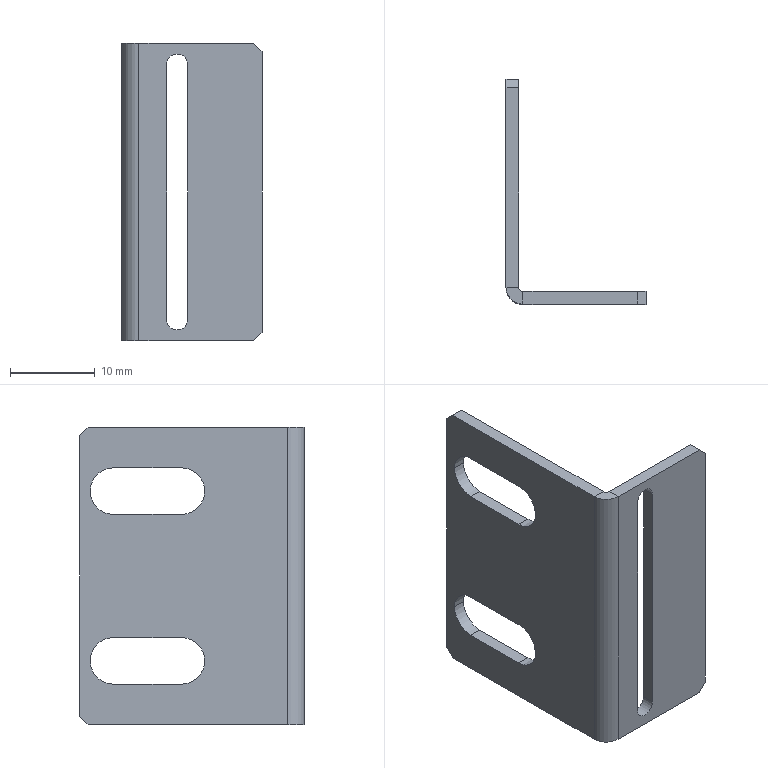Part | SolidWorks | features ICE 2, Chamfer 1, FlatPattern 1, SMBaseFlange 1, SheetMetal 1 | 1 solid | 32 faces | box 16.5 x 26.5 x 35 mm | volume 1824 mm3 | plane 22 | cylinder 10 | commonest cylinder face diameters 5.5 x6 2.5 x2 1 x1 4 x1
STEP:
#1=CARTESIAN_POINT('',(-1.5,23.75,-10.));
#2=VERTEX_POINT('',#1);
#3=CARTESIAN_POINT('',(-1.5,21.,-7.25));
#4=VERTEX_POINT('',#3);
#5=CARTESIAN_POINT('',(-1.5,21.,-10.));
#6=DIRECTION('',(1.,0.,0.));
#7=DIRECTION('',(0.,1.,0.));
#8=AXIS2_PLACEMENT_3D('',#5,#6,#7);
#9=CIRCLE('',#8,2.75);
#10=EDGE_CURVE('',#2,#4,#9,.T.);
#11=ORIENTED_EDGE('',*,*,#10,.F.);
#12=CARTESIAN_POINT('',(0.,23.75,-10.));
#13=VERTEX_POINT('',#12);
#14=CARTESIAN_POINT('',(-10.,23.75,-10.));
#15=DIRECTION('',(1.,0.,0.));
#16=VECTOR('',#15,1000.);
#17=LINE('',#14,#16);
#18=EDGE_CURVE('',#2,#13,#17,.T.);
#19=ORIENTED_EDGE('',*,*,#18,.T.);
#20=CARTESIAN_POINT('',(0.,21.,-7.25));
#21=VERTEX_POINT('',#20);
#22=CARTESIAN_POINT('',(0.,21.,-10.));
#23=DIRECTION('',(1.,0.,0.));
#24=DIRECTION('',(0.,1.,0.));
#25=AXIS2_PLACEMENT_3D('',#22,#23,#24);
#26=CIRCLE('',#25,2.75);
#27=EDGE_CURVE('',#13,#21,#26,.T.);
#28=ORIENTED_EDGE('',*,*,#27,.T.);
#29=CARTESIAN_POINT('',(-10.,21.,-7.25));
#30=DIRECTION('',(1.,0.,0.));
#31=VECTOR('',#30,1000.);
#32=LINE('',#29,#31);
#33=EDGE_CURVE('',#4,#21,#32,.T.);
#34=ORIENTED_EDGE('',*,*,#33,.F.);
#35=EDGE_LOOP('',(#11,#19,#28,#34));
#36=FACE_OUTER_BOUND('',#35,.T.);
#37=CARTESIAN_POINT('',(-10.,21.,-10.));
#38=DIRECTION('',(1.,0.,0.));
#39=DIRECTION('',(0.,1.,0.));
#40=AXIS2_PLACEMENT_3D('',#37,#38,#39);
#41=CYLINDRICAL_SURFACE('',#40,2.75);
#42=ADVANCED_FACE('',(#36),#41,.F.);
#43=CARTESIAN_POINT('',(-1.5,23.75,10.));
#44=VERTEX_POINT('',#43);
#45=CARTESIAN_POINT('',(-1.5,21.,12.75));
#46=VERTEX_POINT('',#45);
#47=CARTESIAN_POINT('',(-1.5,21.,10.));
#48=DIRECTION('',(1.,0.,0.));
#49=DIRECTION('',(0.,1.,0.));
#50=AXIS2_PLACEMENT_3D('',#47,#48,#49);
#51=CIRCLE('',#50,2.75);
#52=EDGE_CURVE('',#44,#46,#51,.T.);
#53=ORIENTED_EDGE('',*,*,#52,.F.);
#54=CARTESIAN_POINT('',(0.,23.75,10.));
#55=VERTEX_POINT('',#54);
#56=CARTESIAN_POINT('',(-10.,23.75,10.));
#57=DIRECTION('',(1.,0.,0.));
#58=VECTOR('',#57,1000.);
#59=LINE('',#56,#58);
#60=EDGE_CURVE('',#44,#55,#59,.T.);
#61=ORIENTED_EDGE('',*,*,#60,.T.);
#62=CARTESIAN_POINT('',(0.,21.,12.75));
#63=VERTEX_POINT('',#62);
#64=CARTESIAN_POINT('',(0.,21.,10.));
#65=DIRECTION('',(1.,0.,0.));
#66=DIRECTION('',(0.,1.,0.));
#67=AXIS2_PLACEMENT_3D('',#64,#65,#66);
#68=CIRCLE('',#67,2.75);
#69=EDGE_CURVE('',#55,#63,#68,.T.);
#70=ORIENTED_EDGE('',*,*,#69,.T.);
#71=CARTESIAN_POINT('',(-10.,21.,12.75));
#72=DIRECTION('',(1.,0.,0.));
#73=VECTOR('',#72,1000.);
#74=LINE('',#71,#73);
#75=EDGE_CURVE('',#46,#63,#74,.T.);
#76=ORIENTED_EDGE('',*,*,#75,.F.);
#77=EDGE_LOOP('',(#53,#61,#70,#76));
#78=FACE_OUTER_BOUND('',#77,.T.);
#79=CARTESIAN_POINT('',(-10.,21.,10.));
#80=DIRECTION('',(1.,0.,0.));
#81=DIRECTION('',(0.,1.,0.));
#82=AXIS2_PLACEMENT_3D('',#79,#80,#81);
#83=CYLINDRICAL_SURFACE('',#82,2.75);
#84=ADVANCED_FACE('',(#78),#83,.F.);
#85=CARTESIAN_POINT('',(0.5,0.,17.5));
#86=VERTEX_POINT('',#85);
#87=CARTESIAN_POINT('',(0.5,-1.5,17.5));
#88=VERTEX_POINT('',#87);
#89=CARTESIAN_POINT('',(0.5,0.,17.5));
#90=DIRECTION('',(0.,-1.,0.));
#91=VECTOR('',#90,1000.);
#92=LINE('',#89,#91);
#93=EDGE_CURVE('',#86,#88,#92,.T.);
#94=ORIENTED_EDGE('',*,*,#93,.F.);
#95=CARTESIAN_POINT('',(0.,0.5,17.5));
#96=VERTEX_POINT('',#95);
#97=CARTESIAN_POINT('',(0.5,0.5,17.5));
#98=DIRECTION('',(0.,0.,1.));
#99=DIRECTION('',(-1.,0.,0.));
#100=AXIS2_PLACEMENT_3D('',#97,#98,#99);
#101=CIRCLE('',#100,0.5);
#102=EDGE_CURVE('',#96,#86,#101,.T.);
#103=ORIENTED_EDGE('',*,*,#102,.F.);
#104=CARTESIAN_POINT('',(-1.5,0.5,17.5));
#105=VERTEX_POINT('',#104);
#106=CARTESIAN_POINT('',(-1.5,0.5,17.5));
#107=DIRECTION('',(1.,0.,0.));
#108=VECTOR('',#107,1000.);
#109=LINE('',#106,#108);
#110=EDGE_CURVE('',#105,#96,#109,.T.);
#111=ORIENTED_EDGE('',*,*,#110,.F.);
#112=CARTESIAN_POINT('',(0.5,0.5,17.5));
#113=DIRECTION('',(0.,0.,1.));
#114=DIRECTION('',(1.,0.,0.));
#115=AXIS2_PLACEMENT_3D('',#112,#113,#114);
#116=CIRCLE('',#115,2.);
#117=EDGE_CURVE('',#105,#88,#116,.T.);
#118=ORIENTED_EDGE('',*,*,#117,.T.);
#119=EDGE_LOOP('',(#94,#103,#111,#118));
#120=FACE_OUTER_BOUND('',#119,.T.);
#121=CARTESIAN_POINT('',(0.5,0.,17.5));
#122=DIRECTION('',(0.,0.,1.));
#123=DIRECTION('',(1.,0.,0.));
#124=AXIS2_PLACEMENT_3D('',#121,#122,#123);
#125=PLANE('',#124);
#126=ADVANCED_FACE('',(#120),#125,.T.);
#127=CARTESIAN_POINT('',(14.,-1.5,17.5));
#128=VERTEX_POINT('',#127);
#129=CARTESIAN_POINT('',(0.,-1.5,17.5));
#130=DIRECTION('',(1.,0.,0.));
#131=VECTOR('',#130,1000.);
#132=LINE('',#129,#131);
#133=EDGE_CURVE('',#88,#128,#132,.T.);
#134=ORIENTED_EDGE('',*,*,#133,.T.);
#135=CARTESIAN_POINT('',(14.,0.,17.5));
#136=VERTEX_POINT('',#135);
#137=CARTESIAN_POINT('',(14.,0.5,17.5));
#138=DIRECTION('',(0.,1.,0.));
#139=VECTOR('',#138,1000.);
#140=LINE('',#137,#139);
#141=EDGE_CURVE('',#128,#136,#140,.T.);
#142=ORIENTED_EDGE('',*,*,#141,.T.);
#143=CARTESIAN_POINT('',(0.,0.,17.5));
#144=DIRECTION('',(1.,0.,0.));
#145=VECTOR('',#144,1000.);
#146=LINE('',#143,#145);
#147=EDGE_CURVE('',#86,#136,#146,.T.);
#148=ORIENTED_EDGE('',*,*,#147,.F.);
#149=ORIENTED_EDGE('',*,*,#93,.T.);
#150=EDGE_LOOP('',(#134,#142,#148,#149));
#151=FACE_OUTER_BOUND('',#150,.T.);
#152=CARTESIAN_POINT('',(-1.5,0.5,17.5));
#153=DIRECTION('',(0.,0.,1.));
#154=DIRECTION('',(1.,0.,0.));
#155=AXIS2_PLACEMENT_3D('',#152,#153,#154);
#156=PLANE('',#155);
#157=ADVANCED_FACE('',(#151),#156,.T.);
#158=CARTESIAN_POINT('',(0.,0.5,-17.5));
#159=VERTEX_POINT('',#158);
#160=CARTESIAN_POINT('',(-1.5,0.5,-17.5));
#161=VERTEX_POINT('',#160);
#162=CARTESIAN_POINT('',(0.,0.5,-17.5));
#163=DIRECTION('',(-1.,0.,0.));
#164=VECTOR('',#163,1000.);
#165=LINE('',#162,#164);
#166=EDGE_CURVE('',#159,#161,#165,.T.);
#167=ORIENTED_EDGE('',*,*,#166,.F.);
#168=CARTESIAN_POINT('',(0.5,0.,-17.5));
#169=VERTEX_POINT('',#168);
#170=CARTESIAN_POINT('',(0.5,0.5,-17.5));
#171=DIRECTION('',(0.,0.,1.));
#172=DIRECTION('',(-1.,0.,0.));
#173=AXIS2_PLACEMENT_3D('',#170,#171,#172);
#174=CIRCLE('',#173,0.5);
#175=EDGE_CURVE('',#159,#169,#174,.T.);
#176=ORIENTED_EDGE('',*,*,#175,.T.);
#177=CARTESIAN_POINT('',(0.5,-1.5,-17.5));
#178=VERTEX_POINT('',#177);
#179=CARTESIAN_POINT('',(0.5,-1.5,-17.5));
#180=DIRECTION('',(0.,1.,0.));
#181=VECTOR('',#180,1000.);
#182=LINE('',#179,#181);
#183=EDGE_CURVE('',#178,#169,#182,.T.);
#184=ORIENTED_EDGE('',*,*,#183,.F.);
#185=CARTESIAN_POINT('',(0.5,0.5,-17.5));
#186=DIRECTION('',(0.,0.,1.));
#187=DIRECTION('',(1.,0.,0.));
#188=AXIS2_PLACEMENT_3D('',#185,#186,#187);
#189=CIRCLE('',#188,2.);
#190=EDGE_CURVE('',#161,#178,#189,.T.);
#191=ORIENTED_EDGE('',*,*,#190,.F.);
#192=EDGE_LOOP('',(#167,#176,#184,#191));
#193=FACE_OUTER_BOUND('',#192,.T.);
#194=CARTESIAN_POINT('',(0.,0.5,-17.5));
#195=DIRECTION('',(0.,0.,-1.));
#196=DIRECTION('',(-1.,0.,0.));
#197=AXIS2_PLACEMENT_3D('',#194,#195,#196);
#198=PLANE('',#197);
#199=ADVANCED_FACE('',(#193),#198,.T.);
#200=CARTESIAN_POINT('',(-1.5,24.,-17.5));
#201=VERTEX_POINT('',#200);
#202=CARTESIAN_POINT('',(-1.5,25.,-17.5));
#203=DIRECTION('',(0.,-1.,0.));
#204=VECTOR('',#203,1000.);
#205=LINE('',#202,#204);
#206=EDGE_CURVE('',#201,#161,#205,.T.);
#207=ORIENTED_EDGE('',*,*,#206,.F.);
#208=CARTESIAN_POINT('',(0.,24.,-17.5));
#209=VERTEX_POINT('',#208);
#210=CARTESIAN_POINT('',(0.5,24.,-17.5));
#211=DIRECTION('',(1.,0.,0.));
#212=VECTOR('',#211,1000.);
#213=LINE('',#210,#212);
#214=EDGE_CURVE('',#201,#209,#213,.T.);
#215=ORIENTED_EDGE('',*,*,#214,.T.);
#216=CARTESIAN_POINT('',(0.,25.,-17.5));
#217=DIRECTION('',(0.,-1.,0.));
#218=VECTOR('',#217,1000.);
#219=LINE('',#216,#218);
#220=EDGE_CURVE('',#209,#159,#219,.T.);
#221=ORIENTED_EDGE('',*,*,#220,.T.);
#222=ORIENTED_EDGE('',*,*,#166,.T.);
#223=EDGE_LOOP('',(#207,#215,#221,#222));
#224=FACE_OUTER_BOUND('',#223,.T.);
#225=CARTESIAN_POINT('',(0.5,-1.5,-17.5));
#226=DIRECTION('',(0.,0.,-1.));
#227=DIRECTION('',(-1.,0.,0.));
#228=AXIS2_PLACEMENT_3D('',#225,#226,#227);
#229=PLANE('',#228);
#230=ADVANCED_FACE('',(#224),#229,.T.);
#231=CARTESIAN_POINT('',(3.75,-1.5,-15.));
#232=VERTEX_POINT('',#231);
#233=CARTESIAN_POINT('',(3.75,-1.5,15.));
#234=VERTEX_POINT('',#233);
#235=CARTESIAN_POINT('',(3.75,-1.5,17.5));
#236=DIRECTION('',(0.,0.,1.));
#237=VECTOR('',#236,1000.);
#238=LINE('',#235,#237);
#239=EDGE_CURVE('',#232,#234,#238,.T.);
#240=ORIENTED_EDGE('',*,*,#239,.T.);
#241=CARTESIAN_POINT('',(6.25,-1.5,15.));
#242=VERTEX_POINT('',#241);
#243=CARTESIAN_POINT('',(5.,-1.5,15.));
#244=DIRECTION('',(0.,1.,0.));
#245=DIRECTION('',(-1.,0.,0.));
#246=AXIS2_PLACEMENT_3D('',#243,#244,#245);
#247=CIRCLE('',#246,1.25);
#248=EDGE_CURVE('',#234,#242,#247,.T.);
#249=ORIENTED_EDGE('',*,*,#248,.T.);
#250=CARTESIAN_POINT('',(6.25,-1.5,-15.));
#251=VERTEX_POINT('',#250);
#252=CARTESIAN_POINT('',(6.25,-1.5,17.5));
#253=DIRECTION('',(0.,0.,-1.));
#254=VECTOR('',#253,1000.);
#255=LINE('',#252,#254);
#256=EDGE_CURVE('',#242,#251,#255,.T.);
#257=ORIENTED_EDGE('',*,*,#256,.T.);
#258=CARTESIAN_POINT('',(5.,-1.5,-15.));
#259=DIRECTION('',(0.,1.,0.));
#260=DIRECTION('',(-1.,0.,0.));
#261=AXIS2_PLACEMENT_3D('',#258,#259,#260);
#262=CIRCLE('',#261,1.25);
#263=EDGE_CURVE('',#251,#232,#262,.T.);
#264=ORIENTED_EDGE('',*,*,#263,.T.);
#265=EDGE_LOOP('',(#240,#249,#257,#264));
#266=FACE_BOUND('',#265,.T.);
#267=CARTESIAN_POINT('',(14.,-1.5,-17.5));
#268=VERTEX_POINT('',#267);
#269=CARTESIAN_POINT('',(0.,-1.5,-17.5));
#270=DIRECTION('',(1.,0.,0.));
#271=VECTOR('',#270,1000.);
#272=LINE('',#269,#271);
#273=EDGE_CURVE('',#178,#268,#272,.T.);
#274=ORIENTED_EDGE('',*,*,#273,.T.);
#275=CARTESIAN_POINT('',(15.,-1.5,-16.5));
#276=VERTEX_POINT('',#275);
#277=CARTESIAN_POINT('',(14.,-1.5,-17.5));
#278=DIRECTION('',(0.7071,0.,0.7071));
#279=VECTOR('',#278,1000.);
#280=LINE('',#277,#279);
#281=EDGE_CURVE('',#268,#276,#280,.T.);
#282=ORIENTED_EDGE('',*,*,#281,.T.);
#283=CARTESIAN_POINT('',(15.,-1.5,16.5));
#284=VERTEX_POINT('',#283);
#285=CARTESIAN_POINT('',(15.,-1.5,17.5));
#286=DIRECTION('',(0.,0.,-1.));
#287=VECTOR('',#286,1000.);
#288=LINE('',#285,#287);
#289=EDGE_CURVE('',#284,#276,#288,.T.);
#290=ORIENTED_EDGE('',*,*,#289,.F.);
#291=CARTESIAN_POINT('',(15.,-1.5,16.5));
#292=DIRECTION('',(-0.7071,0.,0.7071));
#293=VECTOR('',#292,1000.);
#294=LINE('',#291,#293);
#295=EDGE_CURVE('',#284,#128,#294,.T.);
#296=ORIENTED_EDGE('',*,*,#295,.T.);
#297=ORIENTED_EDGE('',*,*,#133,.F.);
#298=CARTESIAN_POINT('',(0.5,-1.5,17.5));
#299=DIRECTION('',(0.,0.,-1.));
#300=VECTOR('',#299,1000.);
#301=LINE('',#298,#300);
#302=EDGE_CURVE('',#88,#178,#301,.T.);
#303=ORIENTED_EDGE('',*,*,#302,.T.);
#304=EDGE_LOOP('',(#274,#282,#290,#296,#297,#303));
#305=FACE_OUTER_BOUND('',#304,.T.);
#306=CARTESIAN_POINT('',(0.,-1.5,17.5));
#307=DIRECTION('',(0.,1.,0.));
#308=DIRECTION('',(-1.,0.,0.));
#309=AXIS2_PLACEMENT_3D('',#306,#307,#308);
#310=PLANE('',#309);
#311=ADVANCED_FACE('',(#266,#305),#310,.F.);
#312=ORIENTED_EDGE('',*,*,#289,.T.);
#313=CARTESIAN_POINT('',(15.,0.,-16.5));
#314=VERTEX_POINT('',#313);
#315=CARTESIAN_POINT('',(15.,0.,-16.5));
#316=DIRECTION('',(0.,1.,0.));
#317=VECTOR('',#316,1000.);
#318=LINE('',#315,#317);
#319=EDGE_CURVE('',#276,#314,#318,.T.);
#320=ORIENTED_EDGE('',*,*,#319,.T.);
#321=CARTESIAN_POINT('',(15.,0.,16.5));
#322=VERTEX_POINT('',#321);
#323=CARTESIAN_POINT('',(15.,0.,17.5));
#324=DIRECTION('',(0.,0.,-1.));
#325=VECTOR('',#324,1000.);
#326=LINE('',#323,#325);
#327=EDGE_CURVE('',#322,#314,#326,.T.);
#328=ORIENTED_EDGE('',*,*,#327,.F.);
#329=CARTESIAN_POINT('',(15.,0.,16.5));
#330=DIRECTION('',(0.,-1.,0.));
#331=VECTOR('',#330,1000.);
#332=LINE('',#329,#331);
#333=EDGE_CURVE('',#322,#284,#332,.T.);
#334=ORIENTED_EDGE('',*,*,#333,.T.);
#335=EDGE_LOOP('',(#312,#320,#328,#334));
#336=FACE_OUTER_BOUND('',#335,.T.);
#337=CARTESIAN_POINT('',(15.,0.,17.5));
#338=DIRECTION('',(1.,0.,0.));
#339=DIRECTION('',(0.,0.,-1.));
#340=AXIS2_PLACEMENT_3D('',#337,#338,#339);
#341=PLANE('',#340);
#342=ADVANCED_FACE('',(#336),#341,.T.);
#343=CARTESIAN_POINT('',(3.75,0.,15.));
#344=VERTEX_POINT('',#343);
#345=CARTESIAN_POINT('',(6.25,0.,15.));
#346=VERTEX_POINT('',#345);
#347=CARTESIAN_POINT('',(5.,0.,15.));
#348=DIRECTION('',(0.,1.,0.));
#349=DIRECTION('',(-1.,0.,0.));
#350=AXIS2_PLACEMENT_3D('',#347,#348,#349);
#351=CIRCLE('',#350,1.25);
#352=EDGE_CURVE('',#344,#346,#351,.T.);
#353=ORIENTED_EDGE('',*,*,#352,.F.);
#354=CARTESIAN_POINT('',(3.75,0.,-15.));
#355=VERTEX_POINT('',#354);
#356=CARTESIAN_POINT('',(3.75,0.,15.));
#357=DIRECTION('',(0.,0.,1.));
#358=VECTOR('',#357,1000.);
#359=LINE('',#356,#358);
#360=EDGE_CURVE('',#355,#344,#359,.T.);
#361=ORIENTED_EDGE('',*,*,#360,.F.);
#362=CARTESIAN_POINT('',(6.25,0.,-15.));
#363=VERTEX_POINT('',#362);
#364=CARTESIAN_POINT('',(5.,0.,-15.));
#365=DIRECTION('',(0.,1.,0.));
#366=DIRECTION('',(-1.,0.,0.));
#367=AXIS2_PLACEMENT_3D('',#364,#365,#366);
#368=CIRCLE('',#367,1.25);
#369=EDGE_CURVE('',#363,#355,#368,.T.);
#370=ORIENTED_EDGE('',*,*,#369,.F.);
#371=CARTESIAN_POINT('',(6.25,0.,15.));
#372=DIRECTION('',(0.,0.,-1.));
#373=VECTOR('',#372,1000.);
#374=LINE('',#371,#373);
#375=EDGE_CURVE('',#346,#363,#374,.T.);
#376=ORIENTED_EDGE('',*,*,#375,.F.);
#377=EDGE_LOOP('',(#353,#361,#370,#376));
#378=FACE_BOUND('',#377,.T.);
#379=ORIENTED_EDGE('',*,*,#327,.T.);
#380=CARTESIAN_POINT('',(14.,0.,-17.5));
#381=VERTEX_POINT('',#380);
#382=CARTESIAN_POINT('',(24.5,0.,-7.));
#383=DIRECTION('',(-0.7071,0.,-0.7071));
#384=VECTOR('',#383,1000.);
#385=LINE('',#382,#384);
#386=EDGE_CURVE('',#314,#381,#385,.T.);
#387=ORIENTED_EDGE('',*,*,#386,.T.);
#388=CARTESIAN_POINT('',(0.,0.,-17.5));
#389=DIRECTION('',(1.,0.,0.));
#390=VECTOR('',#389,1000.);
#391=LINE('',#388,#390);
#392=EDGE_CURVE('',#169,#381,#391,.T.);
#393=ORIENTED_EDGE('',*,*,#392,.F.);
#394=CARTESIAN_POINT('',(0.5,0.,17.5));
#395=DIRECTION('',(0.,0.,-1.));
#396=VECTOR('',#395,1000.);
#397=LINE('',#394,#396);
#398=EDGE_CURVE('',#86,#169,#397,.T.);
#399=ORIENTED_EDGE('',*,*,#398,.F.);
#400=ORIENTED_EDGE('',*,*,#147,.T.);
#401=CARTESIAN_POINT('',(7.,0.,24.5));
#402=DIRECTION('',(0.7071,0.,-0.7071));
#403=VECTOR('',#402,1000.);
#404=LINE('',#401,#403);
#405=EDGE_CURVE('',#136,#322,#404,.T.);
#406=ORIENTED_EDGE('',*,*,#405,.T.);
#407=EDGE_LOOP('',(#379,#387,#393,#399,#400,#406));
#408=FACE_OUTER_BOUND('',#407,.T.);
#409=CARTESIAN_POINT('',(0.,0.,17.5));
#410=DIRECTION('',(0.,1.,0.));
#411=DIRECTION('',(-1.,0.,0.));
#412=AXIS2_PLACEMENT_3D('',#409,#410,#411);
#413=PLANE('',#412);
#414=ADVANCED_FACE('',(#378,#408),#413,.T.);
#415=ORIENTED_EDGE('',*,*,#175,.F.);
#416=CARTESIAN_POINT('',(0.,0.5,17.5));
#417=DIRECTION('',(0.,0.,-1.));
#418=VECTOR('',#417,1000.);
#419=LINE('',#416,#418);
#420=EDGE_CURVE('',#96,#159,#419,.T.);
#421=ORIENTED_EDGE('',*,*,#420,.F.);
#422=ORIENTED_EDGE('',*,*,#102,.T.);
#423=ORIENTED_EDGE('',*,*,#398,.T.);
#424=EDGE_LOOP('',(#415,#421,#422,#423));
#425=FACE_OUTER_BOUND('',#424,.T.);
#426=CARTESIAN_POINT('',(0.5,0.5,17.5));
#427=DIRECTION('',(0.,0.,-1.));
#428=DIRECTION('',(-1.,0.,0.));
#429=AXIS2_PLACEMENT_3D('',#426,#427,#428);
#430=CYLINDRICAL_SURFACE('',#429,0.5);
#431=ADVANCED_FACE('',(#425),#430,.F.);
#432=CARTESIAN_POINT('',(0.,13.,-7.25));
#433=VERTEX_POINT('',#432);
#434=CARTESIAN_POINT('',(0.,13.,-12.75));
#435=VERTEX_POINT('',#434);
#436=CARTESIAN_POINT('',(0.,13.,-10.));
#437=DIRECTION('',(1.,0.,0.));
#438=DIRECTION('',(0.,1.,0.));
#439=AXIS2_PLACEMENT_3D('',#436,#437,#438);
#440=CIRCLE('',#439,2.75);
#441=EDGE_CURVE('',#433,#435,#440,.T.);
#442=ORIENTED_EDGE('',*,*,#441,.F.);
#443=CARTESIAN_POINT('',(0.,13.,-7.25));
#444=DIRECTION('',(0.,-1.,0.));
#445=VECTOR('',#444,1000.);
#446=LINE('',#443,#445);
#447=EDGE_CURVE('',#21,#433,#446,.T.);
#448=ORIENTED_EDGE('',*,*,#447,.F.);
#449=ORIENTED_EDGE('',*,*,#27,.F.);
#450=CARTESIAN_POINT('',(0.,21.,-12.75));
#451=VERTEX_POINT('',#450);
#452=CARTESIAN_POINT('',(0.,21.,-10.));
#453=DIRECTION('',(1.,0.,0.));
#454=DIRECTION('',(0.,1.,0.));
#455=AXIS2_PLACEMENT_3D('',#452,#453,#454);
#456=CIRCLE('',#455,2.75);
#457=EDGE_CURVE('',#451,#13,#456,.T.);
#458=ORIENTED_EDGE('',*,*,#457,.F.);
#459=CARTESIAN_POINT('',(0.,13.,-12.75));
#460=DIRECTION('',(0.,1.,0.));
#461=VECTOR('',#460,1000.);
#462=LINE('',#459,#461);
#463=EDGE_CURVE('',#435,#451,#462,.T.);
#464=ORIENTED_EDGE('',*,*,#463,.F.);
#465=EDGE_LOOP('',(#442,#448,#449,#458,#464));
#466=FACE_BOUND('',#465,.T.);
#467=CARTESIAN_POINT('',(0.,13.,12.75));
#468=VERTEX_POINT('',#467);
#469=CARTESIAN_POINT('',(0.,13.,7.25));
#470=VERTEX_POINT('',#469);
#471=CARTESIAN_POINT('',(0.,13.,10.));
#472=DIRECTION('',(1.,0.,0.));
#473=DIRECTION('',(0.,1.,0.));
#474=AXIS2_PLACEMENT_3D('',#471,#472,#473);
#475=CIRCLE('',#474,2.75);
#476=EDGE_CURVE('',#468,#470,#475,.T.);
#477=ORIENTED_EDGE('',*,*,#476,.F.);
#478=CARTESIAN_POINT('',(0.,13.,12.75));
#479=DIRECTION('',(0.,-1.,0.));
#480=VECTOR('',#479,1000.);
#481=LINE('',#478,#480);
#482=EDGE_CURVE('',#63,#468,#481,.T.);
#483=ORIENTED_EDGE('',*,*,#482,.F.);
#484=ORIENTED_EDGE('',*,*,#69,.F.);
#485=CARTESIAN_POINT('',(0.,21.,7.25));
#486=VERTEX_POINT('',#485);
#487=CARTESIAN_POINT('',(0.,21.,10.));
#488=DIRECTION('',(1.,0.,0.));
#489=DIRECTION('',(0.,1.,0.));
#490=AXIS2_PLACEMENT_3D('',#487,#488,#489);
#491=CIRCLE('',#490,2.75);
#492=EDGE_CURVE('',#486,#55,#491,.T.);
#493=ORIENTED_EDGE('',*,*,#492,.F.);
#494=CARTESIAN_POINT('',(0.,13.,7.25));
#495=DIRECTION('',(0.,1.,0.));
#496=VECTOR('',#495,1000.);
#497=LINE('',#494,#496);
#498=EDGE_CURVE('',#470,#486,#497,.T.);
#499=ORIENTED_EDGE('',*,*,#498,.F.);
#500=EDGE_LOOP('',(#477,#483,#484,#493,#499));
#501=FACE_BOUND('',#500,.T.);
#502=ORIENTED_EDGE('',*,*,#220,.F.);
#503=CARTESIAN_POINT('',(0.,25.,-16.5));
#504=VERTEX_POINT('',#503);
#505=CARTESIAN_POINT('',(0.,42.,0.5));
#506=DIRECTION('',(0.,0.7071,0.7071));
#507=VECTOR('',#506,1000.);
#508=LINE('',#505,#507);
#509=EDGE_CURVE('',#209,#504,#508,.T.);
#510=ORIENTED_EDGE('',*,*,#509,.T.);
#511=CARTESIAN_POINT('',(0.,25.,16.5));
#512=VERTEX_POINT('',#511);
#513=CARTESIAN_POINT('',(0.,25.,17.5));
#514=DIRECTION('',(0.,0.,-1.));
#515=VECTOR('',#514,1000.);
#516=LINE('',#513,#515);
#517=EDGE_CURVE('',#512,#504,#516,.T.);
#518=ORIENTED_EDGE('',*,*,#517,.F.);
#519=CARTESIAN_POINT('',(0.,24.,17.5));
#520=VERTEX_POINT('',#519);
#521=CARTESIAN_POINT('',(0.,24.5,17.));
#522=DIRECTION('',(0.,-0.7071,0.7071));
#523=VECTOR('',#522,1000.);
#524=LINE('',#521,#523);
#525=EDGE_CURVE('',#512,#520,#524,.T.);
#526=ORIENTED_EDGE('',*,*,#525,.T.);
#527=CARTESIAN_POINT('',(0.,25.,17.5));
#528=DIRECTION('',(0.,-1.,0.));
#529=VECTOR('',#528,1000.);
#530=LINE('',#527,#529);
#531=EDGE_CURVE('',#520,#96,#530,.T.);
#532=ORIENTED_EDGE('',*,*,#531,.T.);
#533=ORIENTED_EDGE('',*,*,#420,.T.);
#534=EDGE_LOOP('',(#502,#510,#518,#526,#532,#533));
#535=FACE_OUTER_BOUND('',#534,.T.);
#536=CARTESIAN_POINT('',(0.,25.,17.5));
#537=DIRECTION('',(1.,0.,0.));
#538=DIRECTION('',(0.,1.,0.));
#539=AXIS2_PLACEMENT_3D('',#536,#537,#538);
#540=PLANE('',#539);
#541=ADVANCED_FACE('',(#466,#501,#535),#540,.T.);
#542=ORIENTED_EDGE('',*,*,#517,.T.);
#543=CARTESIAN_POINT('',(-1.5,25.,-16.5));
#544=VERTEX_POINT('',#543);
#545=CARTESIAN_POINT('',(-1.5,25.,-16.5));
#546=DIRECTION('',(-1.,0.,0.));
#547=VECTOR('',#546,1000.);
#548=LINE('',#545,#547);
#549=EDGE_CURVE('',#504,#544,#548,.T.);
#550=ORIENTED_EDGE('',*,*,#549,.T.);
#551=CARTESIAN_POINT('',(-1.5,25.,16.5));
#552=VERTEX_POINT('',#551);
#553=CARTESIAN_POINT('',(-1.5,25.,17.5));
#554=DIRECTION('',(0.,0.,-1.));
#555=VECTOR('',#554,1000.);
#556=LINE('',#553,#555);
#557=EDGE_CURVE('',#552,#544,#556,.T.);
#558=ORIENTED_EDGE('',*,*,#557,.F.);
#559=CARTESIAN_POINT('',(0.,25.,16.5));
#560=DIRECTION('',(1.,0.,0.));
#561=VECTOR('',#560,1000.);
#562=LINE('',#559,#561);
#563=EDGE_CURVE('',#552,#512,#562,.T.);
#564=ORIENTED_EDGE('',*,*,#563,.T.);
#565=EDGE_LOOP('',(#542,#550,#558,#564));
#566=FACE_OUTER_BOUND('',#565,.T.);
#567=CARTESIAN_POINT('',(-1.5,25.,17.5));
#568=DIRECTION('',(0.,1.,0.));
#569=DIRECTION('',(0.,0.,1.));
#570=AXIS2_PLACEMENT_3D('',#567,#568,#569);
#571=PLANE('',#570);
#572=ADVANCED_FACE('',(#566),#571,.T.);
#573=CARTESIAN_POINT('',(-1.5,13.,-7.25));
#574=VERTEX_POINT('',#573);
#575=CARTESIAN_POINT('',(-1.5,25.,-7.25));
#576=DIRECTION('',(0.,-1.,0.));
#577=VECTOR('',#576,1000.);
#578=LINE('',#575,#577);
#579=EDGE_CURVE('',#4,#574,#578,.T.);
#580=ORIENTED_EDGE('',*,*,#579,.T.);
#581=CARTESIAN_POINT('',(-1.5,13.,-12.75));
#582=VERTEX_POINT('',#581);
#583=CARTESIAN_POINT('',(-1.5,13.,-10.));
#584=DIRECTION('',(1.,0.,0.));
#585=DIRECTION('',(0.,1.,0.));
#586=AXIS2_PLACEMENT_3D('',#583,#584,#585);
#587=CIRCLE('',#586,2.75);
#588=EDGE_CURVE('',#574,#582,#587,.T.);
#589=ORIENTED_EDGE('',*,*,#588,.T.);
#590=CARTESIAN_POINT('',(-1.5,21.,-12.75));
#591=VERTEX_POINT('',#590);
#592=CARTESIAN_POINT('',(-1.5,25.,-12.75));
#593=DIRECTION('',(0.,1.,0.));
#594=VECTOR('',#593,1000.);
#595=LINE('',#592,#594);
#596=EDGE_CURVE('',#582,#591,#595,.T.);
#597=ORIENTED_EDGE('',*,*,#596,.T.);
#598=CARTESIAN_POINT('',(-1.5,21.,-10.));
#599=DIRECTION('',(1.,0.,0.));
#600=DIRECTION('',(0.,1.,0.));
#601=AXIS2_PLACEMENT_3D('',#598,#599,#600);
#602=CIRCLE('',#601,2.75);
#603=EDGE_CURVE('',#591,#2,#602,.T.);
#604=ORIENTED_EDGE('',*,*,#603,.T.);
#605=ORIENTED_EDGE('',*,*,#10,.T.);
#606=EDGE_LOOP('',(#580,#589,#597,#604,#605));
#607=FACE_BOUND('',#606,.T.);
#608=CARTESIAN_POINT('',(-1.5,13.,12.75));
#609=VERTEX_POINT('',#608);
#610=CARTESIAN_POINT('',(-1.5,25.,12.75));
#611=DIRECTION('',(0.,-1.,0.));
#612=VECTOR('',#611,1000.);
#613=LINE('',#610,#612);
#614=EDGE_CURVE('',#46,#609,#613,.T.);
#615=ORIENTED_EDGE('',*,*,#614,.T.);
#616=CARTESIAN_POINT('',(-1.5,13.,7.25));
#617=VERTEX_POINT('',#616);
#618=CARTESIAN_POINT('',(-1.5,13.,10.));
#619=DIRECTION('',(1.,0.,0.));
#620=DIRECTION('',(0.,1.,0.));
#621=AXIS2_PLACEMENT_3D('',#618,#619,#620);
#622=CIRCLE('',#621,2.75);
#623=EDGE_CURVE('',#609,#617,#622,.T.);
#624=ORIENTED_EDGE('',*,*,#623,.T.);
#625=CARTESIAN_POINT('',(-1.5,21.,7.25));
#626=VERTEX_POINT('',#625);
#627=CARTESIAN_POINT('',(-1.5,25.,7.25));
#628=DIRECTION('',(0.,1.,0.));
#629=VECTOR('',#628,1000.);
#630=LINE('',#627,#629);
#631=EDGE_CURVE('',#617,#626,#630,.T.);
#632=ORIENTED_EDGE('',*,*,#631,.T.);
#633=CARTESIAN_POINT('',(-1.5,21.,10.));
#634=DIRECTION('',(1.,0.,0.));
#635=DIRECTION('',(0.,1.,0.));
#636=AXIS2_PLACEMENT_3D('',#633,#634,#635);
#637=CIRCLE('',#636,2.75);
#638=EDGE_CURVE('',#626,#44,#637,.T.);
#639=ORIENTED_EDGE('',*,*,#638,.T.);
#640=ORIENTED_EDGE('',*,*,#52,.T.);
#641=EDGE_LOOP('',(#615,#624,#632,#639,#640));
#642=FACE_BOUND('',#641,.T.);
#643=ORIENTED_EDGE('',*,*,#557,.T.);
#644=CARTESIAN_POINT('',(-1.5,24.,-17.5));
#645=DIRECTION('',(0.,-0.7071,-0.7071));
#646=VECTOR('',#645,1000.);
#647=LINE('',#644,#646);
#648=EDGE_CURVE('',#544,#201,#647,.T.);
#649=ORIENTED_EDGE('',*,*,#648,.T.);
#650=ORIENTED_EDGE('',*,*,#206,.T.);
#651=CARTESIAN_POINT('',(-1.5,0.5,17.5));
#652=DIRECTION('',(0.,0.,-1.));
#653=VECTOR('',#652,1000.);
#654=LINE('',#651,#653);
#655=EDGE_CURVE('',#105,#161,#654,.T.);
#656=ORIENTED_EDGE('',*,*,#655,.F.);
#657=CARTESIAN_POINT('',(-1.5,24.,17.5));
#658=VERTEX_POINT('',#657);
#659=CARTESIAN_POINT('',(-1.5,25.,17.5));
#660=DIRECTION('',(0.,-1.,0.));
#661=VECTOR('',#660,1000.);
#662=LINE('',#659,#661);
#663=EDGE_CURVE('',#658,#105,#662,.T.);
#664=ORIENTED_EDGE('',*,*,#663,.F.);
#665=CARTESIAN_POINT('',(-1.5,25.,16.5));
#666=DIRECTION('',(0.,0.7071,-0.7071));
#667=VECTOR('',#666,1000.);
#668=LINE('',#665,#667);
#669=EDGE_CURVE('',#658,#552,#668,.T.);
#670=ORIENTED_EDGE('',*,*,#669,.T.);
#671=EDGE_LOOP('',(#643,#649,#650,#656,#664,#670));
#672=FACE_OUTER_BOUND('',#671,.T.);
#673=CARTESIAN_POINT('',(-1.5,25.,17.5));
#674=DIRECTION('',(1.,0.,0.));
#675=DIRECTION('',(0.,1.,0.));
#676=AXIS2_PLACEMENT_3D('',#673,#674,#675);
#677=PLANE('',#676);
#678=ADVANCED_FACE('',(#607,#642,#672),#677,.F.);
#679=ORIENTED_EDGE('',*,*,#190,.T.);
#680=ORIENTED_EDGE('',*,*,#302,.F.);
#681=ORIENTED_EDGE('',*,*,#117,.F.);
#682=ORIENTED_EDGE('',*,*,#655,.T.);
#683=EDGE_LOOP('',(#679,#680,#681,#682));
#684=FACE_OUTER_BOUND('',#683,.T.);
#685=CARTESIAN_POINT('',(0.5,0.5,17.5));
#686=DIRECTION('',(0.,0.,-1.));
#687=DIRECTION('',(-1.,0.,0.));
#688=AXIS2_PLACEMENT_3D('',#685,#686,#687);
#689=CYLINDRICAL_SURFACE('',#688,2.);
#690=ADVANCED_FACE('',(#684),#689,.T.);
#691=ORIENTED_EDGE('',*,*,#531,.F.);
#692=CARTESIAN_POINT('',(-1.5,24.,17.5));
#693=DIRECTION('',(-1.,0.,0.));
#694=VECTOR('',#693,1000.);
#695=LINE('',#692,#694);
#696=EDGE_CURVE('',#520,#658,#695,.T.);
#697=ORIENTED_EDGE('',*,*,#696,.T.);
#698=ORIENTED_EDGE('',*,*,#663,.T.);
#699=ORIENTED_EDGE('',*,*,#110,.T.);
#700=EDGE_LOOP('',(#691,#697,#698,#699));
#701=FACE_OUTER_BOUND('',#700,.T.);
#702=CARTESIAN_POINT('',(0.5,0.5,17.5));
#703=DIRECTION('',(0.,0.,-1.));
#704=DIRECTION('',(-1.,0.,0.));
#705=AXIS2_PLACEMENT_3D('',#702,#703,#704);
#706=PLANE('',#705);
#707=ADVANCED_FACE('',(#701),#706,.F.);
#708=ORIENTED_EDGE('',*,*,#392,.T.);
#709=CARTESIAN_POINT('',(14.,0.5,-17.5));
#710=DIRECTION('',(0.,-1.,0.));
#711=VECTOR('',#710,1000.);
#712=LINE('',#709,#711);
#713=EDGE_CURVE('',#381,#268,#712,.T.);
#714=ORIENTED_EDGE('',*,*,#713,.T.);
#715=ORIENTED_EDGE('',*,*,#273,.F.);
#716=ORIENTED_EDGE('',*,*,#183,.T.);
#717=EDGE_LOOP('',(#708,#714,#715,#716));
#718=FACE_OUTER_BOUND('',#717,.T.);
#719=CARTESIAN_POINT('',(0.5,0.5,-17.5));
#720=DIRECTION('',(0.,0.,-1.));
#721=DIRECTION('',(-1.,0.,0.));
#722=AXIS2_PLACEMENT_3D('',#719,#720,#721);
#723=PLANE('',#722);
#724=ADVANCED_FACE('',(#718),#723,.T.);
#725=ORIENTED_EDGE('',*,*,#648,.F.);
#726=ORIENTED_EDGE('',*,*,#549,.F.);
#727=ORIENTED_EDGE('',*,*,#509,.F.);
#728=ORIENTED_EDGE('',*,*,#214,.F.);
#729=EDGE_LOOP('',(#725,#726,#727,#728));
#730=FACE_OUTER_BOUND('',#729,.T.);
#731=CARTESIAN_POINT('',(0.5,24.,-17.5));
#732=DIRECTION('',(0.,-0.7071,0.7071));
#733=DIRECTION('',(1.,0.,0.));
#734=AXIS2_PLACEMENT_3D('',#731,#732,#733);
#735=PLANE('',#734);
#736=ADVANCED_FACE('',(#730),#735,.F.);
#737=ORIENTED_EDGE('',*,*,#669,.F.);
#738=ORIENTED_EDGE('',*,*,#696,.F.);
#739=ORIENTED_EDGE('',*,*,#525,.F.);
#740=ORIENTED_EDGE('',*,*,#563,.F.);
#741=EDGE_LOOP('',(#737,#738,#739,#740));
#742=FACE_OUTER_BOUND('',#741,.T.);
#743=CARTESIAN_POINT('',(-1.5,25.,16.5));
#744=DIRECTION('',(0.,0.7071,0.7071));
#745=DIRECTION('',(-1.,0.,0.));
#746=AXIS2_PLACEMENT_3D('',#743,#744,#745);
#747=PLANE('',#746);
#748=ADVANCED_FACE('',(#742),#747,.T.);
#749=ORIENTED_EDGE('',*,*,#386,.F.);
#750=ORIENTED_EDGE('',*,*,#319,.F.);
#751=ORIENTED_EDGE('',*,*,#281,.F.);
#752=ORIENTED_EDGE('',*,*,#713,.F.);
#753=EDGE_LOOP('',(#749,#750,#751,#752));
#754=FACE_OUTER_BOUND('',#753,.T.);
#755=CARTESIAN_POINT('',(14.,0.5,-17.5));
#756=DIRECTION('',(-0.7071,0.,0.7071));
#757=DIRECTION('',(0.,-1.,0.));
#758=AXIS2_PLACEMENT_3D('',#755,#756,#757);
#759=PLANE('',#758);
#760=ADVANCED_FACE('',(#754),#759,.F.);
#761=ORIENTED_EDGE('',*,*,#405,.F.);
#762=ORIENTED_EDGE('',*,*,#141,.F.);
#763=ORIENTED_EDGE('',*,*,#295,.F.);
#764=ORIENTED_EDGE('',*,*,#333,.F.);
#765=EDGE_LOOP('',(#761,#762,#763,#764));
#766=FACE_OUTER_BOUND('',#765,.T.);
#767=CARTESIAN_POINT('',(15.,0.,16.5));
#768=DIRECTION('',(-0.7071,0.,-0.7071));
#769=DIRECTION('',(0.,-1.,0.));
#770=AXIS2_PLACEMENT_3D('',#767,#768,#769);
#771=PLANE('',#770);
#772=ADVANCED_FACE('',(#766),#771,.F.);
#773=CARTESIAN_POINT('',(-10.,13.,12.75));
#774=DIRECTION('',(1.,0.,0.));
#775=VECTOR('',#774,1000.);
#776=LINE('',#773,#775);
#777=EDGE_CURVE('',#609,#468,#776,.T.);
#778=ORIENTED_EDGE('',*,*,#777,.T.);
#779=ORIENTED_EDGE('',*,*,#476,.T.);
#780=CARTESIAN_POINT('',(-10.,13.,7.25));
#781=DIRECTION('',(1.,0.,0.));
#782=VECTOR('',#781,1000.);
#783=LINE('',#780,#782);
#784=EDGE_CURVE('',#617,#470,#783,.T.);
#785=ORIENTED_EDGE('',*,*,#784,.F.);
#786=ORIENTED_EDGE('',*,*,#623,.F.);
#787=EDGE_LOOP('',(#778,#779,#785,#786));
#788=FACE_OUTER_BOUND('',#787,.T.);
#789=CARTESIAN_POINT('',(-10.,13.,10.));
#790=DIRECTION('',(1.,0.,0.));
#791=DIRECTION('',(0.,1.,0.));
#792=AXIS2_PLACEMENT_3D('',#789,#790,#791);
#793=CYLINDRICAL_SURFACE('',#792,2.75);
#794=ADVANCED_FACE('',(#788),#793,.F.);
#795=ORIENTED_EDGE('',*,*,#75,.T.);
#796=ORIENTED_EDGE('',*,*,#482,.T.);
#797=ORIENTED_EDGE('',*,*,#777,.F.);
#798=ORIENTED_EDGE('',*,*,#614,.F.);
#799=EDGE_LOOP('',(#795,#796,#797,#798));
#800=FACE_OUTER_BOUND('',#799,.T.);
#801=CARTESIAN_POINT('',(-10.,13.,12.75));
#802=DIRECTION('',(0.,0.,1.));
#803=DIRECTION('',(0.,-1.,0.));
#804=AXIS2_PLACEMENT_3D('',#801,#802,#803);
#805=PLANE('',#804);
#806=ADVANCED_FACE('',(#800),#805,.F.);
#807=ORIENTED_EDGE('',*,*,#60,.F.);
#808=ORIENTED_EDGE('',*,*,#638,.F.);
#809=CARTESIAN_POINT('',(-10.,21.,7.25));
#810=DIRECTION('',(1.,0.,0.));
#811=VECTOR('',#810,1000.);
#812=LINE('',#809,#811);
#813=EDGE_CURVE('',#626,#486,#812,.T.);
#814=ORIENTED_EDGE('',*,*,#813,.T.);
#815=ORIENTED_EDGE('',*,*,#492,.T.);
#816=EDGE_LOOP('',(#807,#808,#814,#815));
#817=FACE_OUTER_BOUND('',#816,.T.);
#818=CARTESIAN_POINT('',(-10.,21.,10.));
#819=DIRECTION('',(1.,0.,0.));
#820=DIRECTION('',(0.,1.,0.));
#821=AXIS2_PLACEMENT_3D('',#818,#819,#820);
#822=CYLINDRICAL_SURFACE('',#821,2.75);
#823=ADVANCED_FACE('',(#817),#822,.F.);
#824=ORIENTED_EDGE('',*,*,#784,.T.);
#825=ORIENTED_EDGE('',*,*,#498,.T.);
#826=ORIENTED_EDGE('',*,*,#813,.F.);
#827=ORIENTED_EDGE('',*,*,#631,.F.);
#828=EDGE_LOOP('',(#824,#825,#826,#827));
#829=FACE_OUTER_BOUND('',#828,.T.);
#830=CARTESIAN_POINT('',(-10.,13.,7.25));
#831=DIRECTION('',(0.,0.,-1.));
#832=DIRECTION('',(0.,1.,0.));
#833=AXIS2_PLACEMENT_3D('',#830,#831,#832);
#834=PLANE('',#833);
#835=ADVANCED_FACE('',(#829),#834,.F.);
#836=CARTESIAN_POINT('',(-10.,13.,-7.25));
#837=DIRECTION('',(1.,0.,0.));
#838=VECTOR('',#837,1000.);
#839=LINE('',#836,#838);
#840=EDGE_CURVE('',#574,#433,#839,.T.);
#841=ORIENTED_EDGE('',*,*,#840,.T.);
#842=ORIENTED_EDGE('',*,*,#441,.T.);
#843=CARTESIAN_POINT('',(-10.,13.,-12.75));
#844=DIRECTION('',(1.,0.,0.));
#845=VECTOR('',#844,1000.);
#846=LINE('',#843,#845);
#847=EDGE_CURVE('',#582,#435,#846,.T.);
#848=ORIENTED_EDGE('',*,*,#847,.F.);
#849=ORIENTED_EDGE('',*,*,#588,.F.);
#850=EDGE_LOOP('',(#841,#842,#848,#849));
#851=FACE_OUTER_BOUND('',#850,.T.);
#852=CARTESIAN_POINT('',(-10.,13.,-10.));
#853=DIRECTION('',(1.,0.,0.));
#854=DIRECTION('',(0.,1.,0.));
#855=AXIS2_PLACEMENT_3D('',#852,#853,#854);
#856=CYLINDRICAL_SURFACE('',#855,2.75);
#857=ADVANCED_FACE('',(#851),#856,.F.);
#858=ORIENTED_EDGE('',*,*,#33,.T.);
#859=ORIENTED_EDGE('',*,*,#447,.T.);
#860=ORIENTED_EDGE('',*,*,#840,.F.);
#861=ORIENTED_EDGE('',*,*,#579,.F.);
#862=EDGE_LOOP('',(#858,#859,#860,#861));
#863=FACE_OUTER_BOUND('',#862,.T.);
#864=CARTESIAN_POINT('',(-10.,13.,-7.25));
#865=DIRECTION('',(0.,0.,1.));
#866=DIRECTION('',(0.,-1.,0.));
#867=AXIS2_PLACEMENT_3D('',#864,#865,#866);
#868=PLANE('',#867);
#869=ADVANCED_FACE('',(#863),#868,.F.);
#870=ORIENTED_EDGE('',*,*,#18,.F.);
#871=ORIENTED_EDGE('',*,*,#603,.F.);
#872=CARTESIAN_POINT('',(-10.,21.,-12.75));
#873=DIRECTION('',(1.,0.,0.));
#874=VECTOR('',#873,1000.);
#875=LINE('',#872,#874);
#876=EDGE_CURVE('',#591,#451,#875,.T.);
#877=ORIENTED_EDGE('',*,*,#876,.T.);
#878=ORIENTED_EDGE('',*,*,#457,.T.);
#879=EDGE_LOOP('',(#870,#871,#877,#878));
#880=FACE_OUTER_BOUND('',#879,.T.);
#881=CARTESIAN_POINT('',(-10.,21.,-10.));
#882=DIRECTION('',(1.,0.,0.));
#883=DIRECTION('',(0.,1.,0.));
#884=AXIS2_PLACEMENT_3D('',#881,#882,#883);
#885=CYLINDRICAL_SURFACE('',#884,2.75);
#886=ADVANCED_FACE('',(#880),#885,.F.);
#887=ORIENTED_EDGE('',*,*,#847,.T.);
#888=ORIENTED_EDGE('',*,*,#463,.T.);
#889=ORIENTED_EDGE('',*,*,#876,.F.);
#890=ORIENTED_EDGE('',*,*,#596,.F.);
#891=EDGE_LOOP('',(#887,#888,#889,#890));
#892=FACE_OUTER_BOUND('',#891,.T.);
#893=CARTESIAN_POINT('',(-10.,13.,-12.75));
#894=DIRECTION('',(0.,0.,-1.));
#895=DIRECTION('',(0.,1.,0.));
#896=AXIS2_PLACEMENT_3D('',#893,#894,#895);
#897=PLANE('',#896);
#898=ADVANCED_FACE('',(#892),#897,.F.);
#899=CARTESIAN_POINT('',(3.75,-10.,15.));
#900=DIRECTION('',(0.,1.,0.));
#901=VECTOR('',#900,1000.);
#902=LINE('',#899,#901);
#903=EDGE_CURVE('',#234,#344,#902,.T.);
#904=ORIENTED_EDGE('',*,*,#903,.T.);
#905=ORIENTED_EDGE('',*,*,#352,.T.);
#906=CARTESIAN_POINT('',(6.25,-10.,15.));
#907=DIRECTION('',(0.,1.,0.));
#908=VECTOR('',#907,1000.);
#909=LINE('',#906,#908);
#910=EDGE_CURVE('',#242,#346,#909,.T.);
#911=ORIENTED_EDGE('',*,*,#910,.F.);
#912=ORIENTED_EDGE('',*,*,#248,.F.);
#913=EDGE_LOOP('',(#904,#905,#911,#912));
#914=FACE_OUTER_BOUND('',#913,.T.);
#915=CARTESIAN_POINT('',(5.,-10.,15.));
#916=DIRECTION('',(0.,1.,0.));
#917=DIRECTION('',(-1.,0.,0.));
#918=AXIS2_PLACEMENT_3D('',#915,#916,#917);
#919=CYLINDRICAL_SURFACE('',#918,1.25);
#920=ADVANCED_FACE('',(#914),#919,.F.);
#921=CARTESIAN_POINT('',(3.75,-10.,-15.));
#922=DIRECTION('',(0.,1.,0.));
#923=VECTOR('',#922,1000.);
#924=LINE('',#921,#923);
#925=EDGE_CURVE('',#232,#355,#924,.T.);
#926=ORIENTED_EDGE('',*,*,#925,.T.);
#927=ORIENTED_EDGE('',*,*,#360,.T.);
#928=ORIENTED_EDGE('',*,*,#903,.F.);
#929=ORIENTED_EDGE('',*,*,#239,.F.);
#930=EDGE_LOOP('',(#926,#927,#928,#929));
#931=FACE_OUTER_BOUND('',#930,.T.);
#932=CARTESIAN_POINT('',(3.75,-10.,15.));
#933=DIRECTION('',(-1.,0.,0.));
#934=DIRECTION('',(0.,-1.,0.));
#935=AXIS2_PLACEMENT_3D('',#932,#933,#934);
#936=PLANE('',#935);
#937=ADVANCED_FACE('',(#931),#936,.F.);
#938=CARTESIAN_POINT('',(6.25,-10.,-15.));
#939=DIRECTION('',(0.,1.,0.));
#940=VECTOR('',#939,1000.);
#941=LINE('',#938,#940);
#942=EDGE_CURVE('',#251,#363,#941,.T.);
#943=ORIENTED_EDGE('',*,*,#942,.T.);
#944=ORIENTED_EDGE('',*,*,#369,.T.);
#945=ORIENTED_EDGE('',*,*,#925,.F.);
#946=ORIENTED_EDGE('',*,*,#263,.F.);
#947=EDGE_LOOP('',(#943,#944,#945,#946));
#948=FACE_OUTER_BOUND('',#947,.T.);
#949=CARTESIAN_POINT('',(5.,-10.,-15.));
#950=DIRECTION('',(0.,1.,0.));
#951=DIRECTION('',(-1.,0.,0.));
#952=AXIS2_PLACEMENT_3D('',#949,#950,#951);
#953=CYLINDRICAL_SURFACE('',#952,1.25);
#954=ADVANCED_FACE('',(#948),#953,.F.);
#955=ORIENTED_EDGE('',*,*,#910,.T.);
#956=ORIENTED_EDGE('',*,*,#375,.T.);
#957=ORIENTED_EDGE('',*,*,#942,.F.);
#958=ORIENTED_EDGE('',*,*,#256,.F.);
#959=EDGE_LOOP('',(#955,#956,#957,#958));
#960=FACE_OUTER_BOUND('',#959,.T.);
#961=CARTESIAN_POINT('',(6.25,-10.,15.));
#962=DIRECTION('',(1.,0.,0.));
#963=DIRECTION('',(0.,1.,0.));
#964=AXIS2_PLACEMENT_3D('',#961,#962,#963);
#965=PLANE('',#964);
#966=ADVANCED_FACE('',(#960),#965,.F.);
#967=CLOSED_SHELL('',(#42,#84,#126,#157,#199,#230,#311,#342,#414,#431,#541,#572,#678,#690,#707,#724,#736,#748,#760,#772,#794,#806,#823,#835,#857,#869,#886,#898,#920,#937,#954,#966));
#968=MANIFOLD_SOLID_BREP('',#967);
#969=CARTESIAN_POINT('',(0.,0.,0.));
#970=DIRECTION('',(0.,0.,1.));
#971=DIRECTION('',(1.,0.,0.));
#972=AXIS2_PLACEMENT_3D('',#969,#970,#971);
#973=(LENGTH_UNIT()NAMED_UNIT(*)SI_UNIT(.MILLI.,.METRE.));
#974=UNCERTAINTY_MEASURE_WITH_UNIT(LENGTH_MEASURE(0.00001),#973,'','');
#975=(NAMED_UNIT(*)PLANE_ANGLE_UNIT()SI_UNIT($,.RADIAN.));
#976=(NAMED_UNIT(*)SI_UNIT($,.STERADIAN.)SOLID_ANGLE_UNIT());
#977=(GEOMETRIC_REPRESENTATION_CONTEXT(3)GLOBAL_UNCERTAINTY_ASSIGNED_CONTEXT((#974))GLOBAL_UNIT_ASSIGNED_CONTEXT((#973,#975,#976))REPRESENTATION_CONTEXT('',''));
#978=ADVANCED_BREP_SHAPE_REPRESENTATION('',(#968,#972),#977);